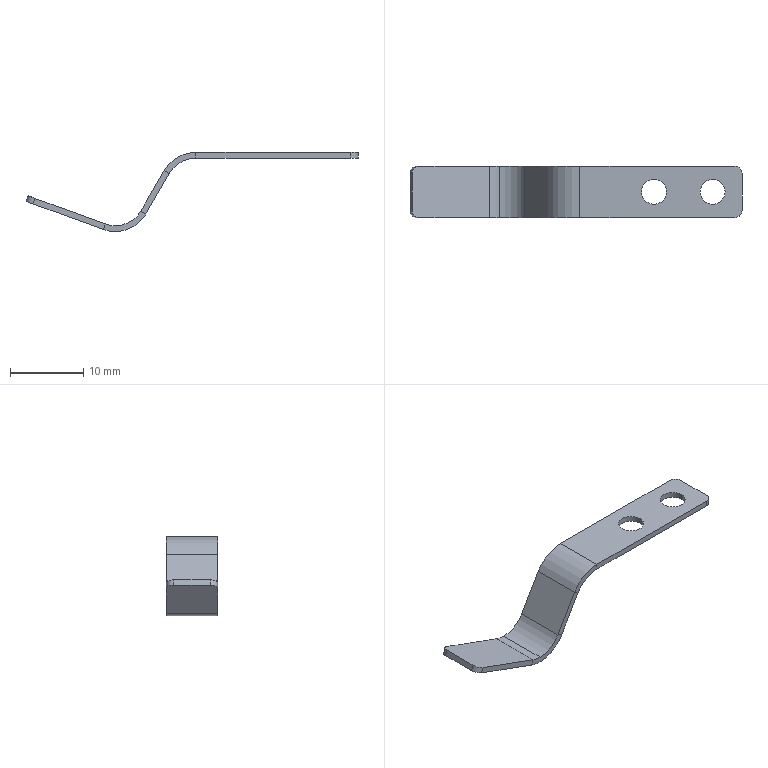Part | NX | features BREP 1 | 1 solid | 32 faces | box 45.274 x 7 x 10.8 mm | volume 268.431 mm3 | plane 18 | cylinder 14 | commonest cylinder face diameters 2 x4 3.4 x4 8 x2 9.6 x2 8.4 x1 10 x1
STEP:
#1=CARTESIAN_POINT('',(-2.3,0.,0.));
#2=VERTEX_POINT('',#1);
#3=CARTESIAN_POINT('',(-5.7,0.,0.));
#4=VERTEX_POINT('',#3);
#5=CARTESIAN_POINT('',(-4.,0.,0.));
#6=DIRECTION('',(0.,0.,-1.));
#7=DIRECTION('',(-1.,0.,0.));
#8=AXIS2_PLACEMENT_3D('',#5,#6,#7);
#9=CIRCLE('',#8,1.7);
#10=EDGE_CURVE('',#2,#4,#9,.T.);
#11=ORIENTED_EDGE('',*,*,#10,.F.);
#12=CARTESIAN_POINT('',(-2.3,0.,-0.8));
#13=VERTEX_POINT('',#12);
#14=CARTESIAN_POINT('',(-2.3,0.,-0.8));
#15=DIRECTION('',(0.,0.,-1.));
#16=VECTOR('',#15,1000.);
#17=LINE('',#14,#16);
#18=EDGE_CURVE('',#13,#2,#17,.F.);
#19=ORIENTED_EDGE('',*,*,#18,.F.);
#20=CARTESIAN_POINT('',(-5.7,0.,-0.8));
#21=VERTEX_POINT('',#20);
#22=CARTESIAN_POINT('',(-4.,0.,-0.8));
#23=DIRECTION('',(0.,0.,-1.));
#24=DIRECTION('',(-1.,0.,0.));
#25=AXIS2_PLACEMENT_3D('',#22,#23,#24);
#26=CIRCLE('',#25,1.7);
#27=EDGE_CURVE('',#13,#21,#26,.T.);
#28=ORIENTED_EDGE('',*,*,#27,.T.);
#29=CARTESIAN_POINT('',(-5.7,0.,-0.8));
#30=DIRECTION('',(0.,0.,-1.));
#31=VECTOR('',#30,1000.);
#32=LINE('',#29,#31);
#33=EDGE_CURVE('',#21,#4,#32,.F.);
#34=ORIENTED_EDGE('',*,*,#33,.T.);
#35=EDGE_LOOP('',(#11,#19,#28,#34));
#36=FACE_BOUND('',#35,.T.);
#37=CARTESIAN_POINT('',(-4.,0.,-0.8));
#38=DIRECTION('',(0.,0.,-1.));
#39=DIRECTION('',(1.,0.,0.));
#40=AXIS2_PLACEMENT_3D('',#37,#38,#39);
#41=CYLINDRICAL_SURFACE('',#40,1.7);
#42=ADVANCED_FACE('',(#36),#41,.F.);
#43=CARTESIAN_POINT('',(-10.3,0.,0.));
#44=VERTEX_POINT('',#43);
#45=CARTESIAN_POINT('',(-13.7,0.,0.));
#46=VERTEX_POINT('',#45);
#47=CARTESIAN_POINT('',(-12.,0.,0.));
#48=DIRECTION('',(0.,0.,-1.));
#49=DIRECTION('',(-1.,0.,0.));
#50=AXIS2_PLACEMENT_3D('',#47,#48,#49);
#51=CIRCLE('',#50,1.7);
#52=EDGE_CURVE('',#44,#46,#51,.T.);
#53=ORIENTED_EDGE('',*,*,#52,.F.);
#54=CARTESIAN_POINT('',(-10.3,0.,-0.8));
#55=VERTEX_POINT('',#54);
#56=CARTESIAN_POINT('',(-10.3,0.,-0.8));
#57=DIRECTION('',(0.,0.,-1.));
#58=VECTOR('',#57,1000.);
#59=LINE('',#56,#58);
#60=EDGE_CURVE('',#55,#44,#59,.F.);
#61=ORIENTED_EDGE('',*,*,#60,.F.);
#62=CARTESIAN_POINT('',(-13.7,0.,-0.8));
#63=VERTEX_POINT('',#62);
#64=CARTESIAN_POINT('',(-12.,0.,-0.8));
#65=DIRECTION('',(0.,0.,-1.));
#66=DIRECTION('',(-1.,0.,0.));
#67=AXIS2_PLACEMENT_3D('',#64,#65,#66);
#68=CIRCLE('',#67,1.7);
#69=EDGE_CURVE('',#55,#63,#68,.T.);
#70=ORIENTED_EDGE('',*,*,#69,.T.);
#71=CARTESIAN_POINT('',(-13.7,0.,-0.8));
#72=DIRECTION('',(0.,0.,-1.));
#73=VECTOR('',#72,1000.);
#74=LINE('',#71,#73);
#75=EDGE_CURVE('',#63,#46,#74,.F.);
#76=ORIENTED_EDGE('',*,*,#75,.T.);
#77=EDGE_LOOP('',(#53,#61,#70,#76));
#78=FACE_BOUND('',#77,.T.);
#79=CARTESIAN_POINT('',(-12.,0.,-0.8));
#80=DIRECTION('',(0.,0.,-1.));
#81=DIRECTION('',(1.,0.,0.));
#82=AXIS2_PLACEMENT_3D('',#79,#80,#81);
#83=CYLINDRICAL_SURFACE('',#82,1.7);
#84=ADVANCED_FACE('',(#78),#83,.F.);
#85=CARTESIAN_POINT('',(-33.083,3.5,-10.8));
#86=VERTEX_POINT('',#85);
#87=CARTESIAN_POINT('',(-34.725,3.5,-10.511));
#88=VERTEX_POINT('',#87);
#89=CARTESIAN_POINT('',(-33.083,3.5,-6.));
#90=DIRECTION('',(0.,1.,0.));
#91=DIRECTION('',(1.,0.,0.));
#92=AXIS2_PLACEMENT_3D('',#89,#90,#91);
#93=CIRCLE('',#92,4.8);
#94=EDGE_CURVE('',#86,#88,#93,.T.);
#95=ORIENTED_EDGE('',*,*,#94,.F.);
#96=CARTESIAN_POINT('',(-33.083,-3.5,-10.8));
#97=VERTEX_POINT('',#96);
#98=CARTESIAN_POINT('',(-33.083,3.5,-10.8));
#99=DIRECTION('',(0.,-1.,0.));
#100=VECTOR('',#99,1000.);
#101=LINE('',#98,#100);
#102=EDGE_CURVE('',#86,#97,#101,.T.);
#103=ORIENTED_EDGE('',*,*,#102,.T.);
#104=CARTESIAN_POINT('',(-34.725,-3.5,-10.511));
#105=VERTEX_POINT('',#104);
#106=CARTESIAN_POINT('',(-33.083,-3.5,-6.));
#107=DIRECTION('',(0.,1.,0.));
#108=DIRECTION('',(1.,0.,0.));
#109=AXIS2_PLACEMENT_3D('',#106,#107,#108);
#110=CIRCLE('',#109,4.8);
#111=EDGE_CURVE('',#97,#105,#110,.T.);
#112=ORIENTED_EDGE('',*,*,#111,.T.);
#113=CARTESIAN_POINT('',(-34.725,3.5,-10.511));
#114=DIRECTION('',(0.,-1.,0.));
#115=VECTOR('',#114,1000.);
#116=LINE('',#113,#115);
#117=EDGE_CURVE('',#88,#105,#116,.T.);
#118=ORIENTED_EDGE('',*,*,#117,.F.);
#119=EDGE_LOOP('',(#95,#103,#112,#118));
#120=FACE_BOUND('',#119,.T.);
#121=CARTESIAN_POINT('',(-33.083,3.5,-6.));
#122=DIRECTION('',(0.,-1.,0.));
#123=DIRECTION('',(0.,0.,1.));
#124=AXIS2_PLACEMENT_3D('',#121,#122,#123);
#125=CYLINDRICAL_SURFACE('',#124,4.8);
#126=ADVANCED_FACE('',(#120),#125,.T.);
#127=CARTESIAN_POINT('',(-29.619,3.5,-8.));
#128=VERTEX_POINT('',#127);
#129=CARTESIAN_POINT('',(-33.083,3.5,-10.));
#130=VERTEX_POINT('',#129);
#131=CARTESIAN_POINT('',(-33.083,3.5,-6.));
#132=DIRECTION('',(0.,1.,0.));
#133=DIRECTION('',(0.,0.,-1.));
#134=AXIS2_PLACEMENT_3D('',#131,#132,#133);
#135=CIRCLE('',#134,4.);
#136=EDGE_CURVE('',#128,#130,#135,.T.);
#137=ORIENTED_EDGE('',*,*,#136,.T.);
#138=CARTESIAN_POINT('',(-33.083,-3.5,-10.));
#139=VERTEX_POINT('',#138);
#140=CARTESIAN_POINT('',(-33.083,3.5,-10.));
#141=DIRECTION('',(0.,-1.,0.));
#142=VECTOR('',#141,1000.);
#143=LINE('',#140,#142);
#144=EDGE_CURVE('',#130,#139,#143,.T.);
#145=ORIENTED_EDGE('',*,*,#144,.T.);
#146=CARTESIAN_POINT('',(-29.619,-3.5,-8.));
#147=VERTEX_POINT('',#146);
#148=CARTESIAN_POINT('',(-33.083,-3.5,-6.));
#149=DIRECTION('',(0.,1.,0.));
#150=DIRECTION('',(0.,0.,-1.));
#151=AXIS2_PLACEMENT_3D('',#148,#149,#150);
#152=CIRCLE('',#151,4.);
#153=EDGE_CURVE('',#147,#139,#152,.T.);
#154=ORIENTED_EDGE('',*,*,#153,.F.);
#155=CARTESIAN_POINT('',(-29.619,3.5,-8.));
#156=DIRECTION('',(0.,-1.,0.));
#157=VECTOR('',#156,1000.);
#158=LINE('',#155,#157);
#159=EDGE_CURVE('',#128,#147,#158,.T.);
#160=ORIENTED_EDGE('',*,*,#159,.F.);
#161=EDGE_LOOP('',(#137,#145,#154,#160));
#162=FACE_BOUND('',#161,.T.);
#163=CARTESIAN_POINT('',(-33.083,3.5,-6.));
#164=DIRECTION('',(0.,-1.,0.));
#165=DIRECTION('',(0.,0.,1.));
#166=AXIS2_PLACEMENT_3D('',#163,#164,#165);
#167=CYLINDRICAL_SURFACE('',#166,4.);
#168=ADVANCED_FACE('',(#162),#167,.F.);
#169=CARTESIAN_POINT('',(-26.443,3.5,-2.5));
#170=VERTEX_POINT('',#169);
#171=CARTESIAN_POINT('',(-25.751,3.5,-2.9));
#172=VERTEX_POINT('',#171);
#173=CARTESIAN_POINT('',(-26.443,3.5,-2.5));
#174=DIRECTION('',(0.866,0.,-0.5));
#175=VECTOR('',#174,1000.);
#176=LINE('',#173,#175);
#177=EDGE_CURVE('',#170,#172,#176,.T.);
#178=ORIENTED_EDGE('',*,*,#177,.F.);
#179=CARTESIAN_POINT('',(-22.113,3.5,0.));
#180=VERTEX_POINT('',#179);
#181=CARTESIAN_POINT('',(-22.113,3.5,-5.));
#182=DIRECTION('',(0.,-1.,0.));
#183=DIRECTION('',(0.,0.,-1.));
#184=AXIS2_PLACEMENT_3D('',#181,#182,#183);
#185=CIRCLE('',#184,5.);
#186=EDGE_CURVE('',#180,#170,#185,.T.);
#187=ORIENTED_EDGE('',*,*,#186,.F.);
#188=CARTESIAN_POINT('',(-22.113,3.5,-0.8));
#189=VERTEX_POINT('',#188);
#190=CARTESIAN_POINT('',(-22.113,3.5,-0.8));
#191=DIRECTION('',(0.,0.,1.));
#192=VECTOR('',#191,1000.);
#193=LINE('',#190,#192);
#194=EDGE_CURVE('',#189,#180,#193,.T.);
#195=ORIENTED_EDGE('',*,*,#194,.F.);
#196=CARTESIAN_POINT('',(-22.113,3.5,-5.));
#197=DIRECTION('',(0.,-1.,0.));
#198=DIRECTION('',(1.,0.,0.));
#199=AXIS2_PLACEMENT_3D('',#196,#197,#198);
#200=CIRCLE('',#199,4.2);
#201=EDGE_CURVE('',#189,#172,#200,.T.);
#202=ORIENTED_EDGE('',*,*,#201,.T.);
#203=EDGE_LOOP('',(#178,#187,#195,#202));
#204=FACE_BOUND('',#203,.T.);
#205=CARTESIAN_POINT('',(-26.443,3.5,-2.5));
#206=DIRECTION('',(0.,1.,0.));
#207=DIRECTION('',(0.,0.,-1.));
#208=AXIS2_PLACEMENT_3D('',#205,#206,#207);
#209=PLANE('',#208);
#210=ADVANCED_FACE('',(#204),#209,.T.);
#211=CARTESIAN_POINT('',(-26.443,3.5,-2.5));
#212=DIRECTION('',(-0.5,0.,-0.866));
#213=VECTOR('',#212,1000.);
#214=LINE('',#211,#213);
#215=EDGE_CURVE('',#170,#128,#214,.T.);
#216=ORIENTED_EDGE('',*,*,#215,.F.);
#217=ORIENTED_EDGE('',*,*,#177,.T.);
#218=CARTESIAN_POINT('',(-28.926,3.5,-8.4));
#219=VERTEX_POINT('',#218);
#220=CARTESIAN_POINT('',(-25.751,3.5,-2.9));
#221=DIRECTION('',(-0.5,0.,-0.866));
#222=VECTOR('',#221,1000.);
#223=LINE('',#220,#222);
#224=EDGE_CURVE('',#172,#219,#223,.T.);
#225=ORIENTED_EDGE('',*,*,#224,.T.);
#226=CARTESIAN_POINT('',(-28.926,3.5,-8.4));
#227=DIRECTION('',(-0.866,0.,0.5));
#228=VECTOR('',#227,1000.);
#229=LINE('',#226,#228);
#230=EDGE_CURVE('',#219,#128,#229,.T.);
#231=ORIENTED_EDGE('',*,*,#230,.T.);
#232=EDGE_LOOP('',(#216,#217,#225,#231));
#233=FACE_BOUND('',#232,.T.);
#234=CARTESIAN_POINT('',(-22.113,3.5,-0.8));
#235=DIRECTION('',(0.,1.,0.));
#236=DIRECTION('',(0.,0.,-1.));
#237=AXIS2_PLACEMENT_3D('',#234,#235,#236);
#238=PLANE('',#237);
#239=ADVANCED_FACE('',(#233),#238,.T.);
#240=CARTESIAN_POINT('',(-22.113,-3.5,0.));
#241=VERTEX_POINT('',#240);
#242=CARTESIAN_POINT('',(-22.113,-3.5,-0.8));
#243=VERTEX_POINT('',#242);
#244=CARTESIAN_POINT('',(-22.113,-3.5,0.));
#245=DIRECTION('',(0.,0.,-1.));
#246=VECTOR('',#245,1000.);
#247=LINE('',#244,#246);
#248=EDGE_CURVE('',#241,#243,#247,.T.);
#249=ORIENTED_EDGE('',*,*,#248,.F.);
#250=CARTESIAN_POINT('',(-26.443,-3.5,-2.5));
#251=VERTEX_POINT('',#250);
#252=CARTESIAN_POINT('',(-22.113,-3.5,-5.));
#253=DIRECTION('',(0.,-1.,0.));
#254=DIRECTION('',(0.,0.,-1.));
#255=AXIS2_PLACEMENT_3D('',#252,#253,#254);
#256=CIRCLE('',#255,5.);
#257=EDGE_CURVE('',#241,#251,#256,.T.);
#258=ORIENTED_EDGE('',*,*,#257,.T.);
#259=CARTESIAN_POINT('',(-25.751,-3.5,-2.9));
#260=VERTEX_POINT('',#259);
#261=CARTESIAN_POINT('',(-25.751,-3.5,-2.9));
#262=DIRECTION('',(-0.866,0.,0.5));
#263=VECTOR('',#262,1000.);
#264=LINE('',#261,#263);
#265=EDGE_CURVE('',#260,#251,#264,.T.);
#266=ORIENTED_EDGE('',*,*,#265,.F.);
#267=CARTESIAN_POINT('',(-22.113,-3.5,-5.));
#268=DIRECTION('',(0.,-1.,0.));
#269=DIRECTION('',(1.,0.,0.));
#270=AXIS2_PLACEMENT_3D('',#267,#268,#269);
#271=CIRCLE('',#270,4.2);
#272=EDGE_CURVE('',#243,#260,#271,.T.);
#273=ORIENTED_EDGE('',*,*,#272,.F.);
#274=EDGE_LOOP('',(#249,#258,#266,#273));
#275=FACE_BOUND('',#274,.T.);
#276=CARTESIAN_POINT('',(-22.113,-3.5,0.));
#277=DIRECTION('',(0.,-1.,0.));
#278=DIRECTION('',(0.,0.,1.));
#279=AXIS2_PLACEMENT_3D('',#276,#277,#278);
#280=PLANE('',#279);
#281=ADVANCED_FACE('',(#275),#280,.T.);
#282=CARTESIAN_POINT('',(-1.,-3.5,-0.8));
#283=VERTEX_POINT('',#282);
#284=CARTESIAN_POINT('',(0.,-3.5,-0.8));
#285=DIRECTION('',(-1.,0.,0.));
#286=VECTOR('',#285,1000.);
#287=LINE('',#284,#286);
#288=EDGE_CURVE('',#283,#243,#287,.T.);
#289=ORIENTED_EDGE('',*,*,#288,.F.);
#290=CARTESIAN_POINT('',(-1.,-3.5,0.));
#291=VERTEX_POINT('',#290);
#292=CARTESIAN_POINT('',(-1.,-3.5,-2.9));
#293=DIRECTION('',(0.,0.,1.));
#294=VECTOR('',#293,1000.);
#295=LINE('',#292,#294);
#296=EDGE_CURVE('',#283,#291,#295,.T.);
#297=ORIENTED_EDGE('',*,*,#296,.T.);
#298=CARTESIAN_POINT('',(0.,-3.5,0.));
#299=DIRECTION('',(-1.,0.,0.));
#300=VECTOR('',#299,1000.);
#301=LINE('',#298,#300);
#302=EDGE_CURVE('',#291,#241,#301,.T.);
#303=ORIENTED_EDGE('',*,*,#302,.T.);
#304=ORIENTED_EDGE('',*,*,#248,.T.);
#305=EDGE_LOOP('',(#289,#297,#303,#304));
#306=FACE_BOUND('',#305,.T.);
#307=CARTESIAN_POINT('',(-25.751,-3.5,-2.9));
#308=DIRECTION('',(0.,-1.,0.));
#309=DIRECTION('',(0.,0.,1.));
#310=AXIS2_PLACEMENT_3D('',#307,#308,#309);
#311=PLANE('',#310);
#312=ADVANCED_FACE('',(#306),#311,.T.);
#313=CARTESIAN_POINT('',(-34.451,3.5,-9.759));
#314=VERTEX_POINT('',#313);
#315=CARTESIAN_POINT('',(-34.451,3.5,-9.759));
#316=DIRECTION('',(-0.342,0.,-0.9397));
#317=VECTOR('',#316,1000.);
#318=LINE('',#315,#317);
#319=EDGE_CURVE('',#314,#88,#318,.T.);
#320=ORIENTED_EDGE('',*,*,#319,.F.);
#321=CARTESIAN_POINT('',(-33.083,3.5,-6.));
#322=DIRECTION('',(0.,1.,0.));
#323=DIRECTION('',(0.,0.,-1.));
#324=AXIS2_PLACEMENT_3D('',#321,#322,#323);
#325=CIRCLE('',#324,4.);
#326=EDGE_CURVE('',#130,#314,#325,.T.);
#327=ORIENTED_EDGE('',*,*,#326,.F.);
#328=ORIENTED_EDGE('',*,*,#136,.F.);
#329=ORIENTED_EDGE('',*,*,#230,.F.);
#330=CARTESIAN_POINT('',(-33.083,3.5,-6.));
#331=DIRECTION('',(0.,1.,0.));
#332=DIRECTION('',(1.,0.,0.));
#333=AXIS2_PLACEMENT_3D('',#330,#331,#332);
#334=CIRCLE('',#333,4.8);
#335=EDGE_CURVE('',#219,#86,#334,.T.);
#336=ORIENTED_EDGE('',*,*,#335,.T.);
#337=ORIENTED_EDGE('',*,*,#94,.T.);
#338=EDGE_LOOP('',(#320,#327,#328,#329,#336,#337));
#339=FACE_BOUND('',#338,.T.);
#340=CARTESIAN_POINT('',(-34.451,3.5,-9.759));
#341=DIRECTION('',(0.,1.,0.));
#342=DIRECTION('',(0.,0.,-1.));
#343=AXIS2_PLACEMENT_3D('',#340,#341,#342);
#344=PLANE('',#343);
#345=ADVANCED_FACE('',(#339),#344,.T.);
#346=CARTESIAN_POINT('',(-44.334,3.5,-7.013));
#347=VERTEX_POINT('',#346);
#348=CARTESIAN_POINT('',(-34.725,3.5,-10.511));
#349=DIRECTION('',(-0.9397,0.,0.342));
#350=VECTOR('',#349,1000.);
#351=LINE('',#348,#350);
#352=EDGE_CURVE('',#88,#347,#351,.T.);
#353=ORIENTED_EDGE('',*,*,#352,.T.);
#354=CARTESIAN_POINT('',(-44.06,3.5,-6.261));
#355=VERTEX_POINT('',#354);
#356=CARTESIAN_POINT('',(-42.977,3.5,-3.286));
#357=DIRECTION('',(0.342,0.,0.9397));
#358=VECTOR('',#357,1000.);
#359=LINE('',#356,#358);
#360=EDGE_CURVE('',#347,#355,#359,.T.);
#361=ORIENTED_EDGE('',*,*,#360,.T.);
#362=CARTESIAN_POINT('',(-34.451,3.5,-9.759));
#363=DIRECTION('',(-0.9397,0.,0.342));
#364=VECTOR('',#363,1000.);
#365=LINE('',#362,#364);
#366=EDGE_CURVE('',#314,#355,#365,.T.);
#367=ORIENTED_EDGE('',*,*,#366,.F.);
#368=ORIENTED_EDGE('',*,*,#319,.T.);
#369=EDGE_LOOP('',(#353,#361,#367,#368));
#370=FACE_BOUND('',#369,.T.);
#371=CARTESIAN_POINT('',(-28.926,3.5,-8.4));
#372=DIRECTION('',(0.,1.,0.));
#373=DIRECTION('',(0.,0.,-1.));
#374=AXIS2_PLACEMENT_3D('',#371,#372,#373);
#375=PLANE('',#374);
#376=ADVANCED_FACE('',(#370),#375,.T.);
#377=CARTESIAN_POINT('',(-28.926,-3.5,-8.4));
#378=VERTEX_POINT('',#377);
#379=CARTESIAN_POINT('',(-29.619,-3.5,-8.));
#380=DIRECTION('',(0.866,0.,-0.5));
#381=VECTOR('',#380,1000.);
#382=LINE('',#379,#381);
#383=EDGE_CURVE('',#147,#378,#382,.T.);
#384=ORIENTED_EDGE('',*,*,#383,.F.);
#385=ORIENTED_EDGE('',*,*,#153,.T.);
#386=CARTESIAN_POINT('',(-34.451,-3.5,-9.759));
#387=VERTEX_POINT('',#386);
#388=CARTESIAN_POINT('',(-33.083,-3.5,-6.));
#389=DIRECTION('',(0.,1.,0.));
#390=DIRECTION('',(0.,0.,-1.));
#391=AXIS2_PLACEMENT_3D('',#388,#389,#390);
#392=CIRCLE('',#391,4.);
#393=EDGE_CURVE('',#139,#387,#392,.T.);
#394=ORIENTED_EDGE('',*,*,#393,.T.);
#395=CARTESIAN_POINT('',(-34.725,-3.5,-10.511));
#396=DIRECTION('',(0.342,0.,0.9397));
#397=VECTOR('',#396,1000.);
#398=LINE('',#395,#397);
#399=EDGE_CURVE('',#105,#387,#398,.T.);
#400=ORIENTED_EDGE('',*,*,#399,.F.);
#401=ORIENTED_EDGE('',*,*,#111,.F.);
#402=CARTESIAN_POINT('',(-33.083,-3.5,-6.));
#403=DIRECTION('',(0.,1.,0.));
#404=DIRECTION('',(1.,0.,0.));
#405=AXIS2_PLACEMENT_3D('',#402,#403,#404);
#406=CIRCLE('',#405,4.8);
#407=EDGE_CURVE('',#378,#97,#406,.T.);
#408=ORIENTED_EDGE('',*,*,#407,.F.);
#409=EDGE_LOOP('',(#384,#385,#394,#400,#401,#408));
#410=FACE_BOUND('',#409,.T.);
#411=CARTESIAN_POINT('',(-29.619,-3.5,-8.));
#412=DIRECTION('',(0.,-1.,0.));
#413=DIRECTION('',(0.,0.,1.));
#414=AXIS2_PLACEMENT_3D('',#411,#412,#413);
#415=PLANE('',#414);
#416=ADVANCED_FACE('',(#410),#415,.T.);
#417=CARTESIAN_POINT('',(-26.443,-3.5,-2.5));
#418=DIRECTION('',(-0.5,0.,-0.866));
#419=VECTOR('',#418,1000.);
#420=LINE('',#417,#419);
#421=EDGE_CURVE('',#251,#147,#420,.T.);
#422=ORIENTED_EDGE('',*,*,#421,.T.);
#423=ORIENTED_EDGE('',*,*,#383,.T.);
#424=CARTESIAN_POINT('',(-25.751,-3.5,-2.9));
#425=DIRECTION('',(-0.5,0.,-0.866));
#426=VECTOR('',#425,1000.);
#427=LINE('',#424,#426);
#428=EDGE_CURVE('',#260,#378,#427,.T.);
#429=ORIENTED_EDGE('',*,*,#428,.F.);
#430=ORIENTED_EDGE('',*,*,#265,.T.);
#431=EDGE_LOOP('',(#422,#423,#429,#430));
#432=FACE_BOUND('',#431,.T.);
#433=CARTESIAN_POINT('',(-34.725,-3.5,-10.511));
#434=DIRECTION('',(0.,-1.,0.));
#435=DIRECTION('',(0.,0.,1.));
#436=AXIS2_PLACEMENT_3D('',#433,#434,#435);
#437=PLANE('',#436);
#438=ADVANCED_FACE('',(#432),#437,.T.);
#439=CARTESIAN_POINT('',(-44.334,-3.5,-7.013));
#440=VERTEX_POINT('',#439);
#441=CARTESIAN_POINT('',(-34.725,-3.5,-10.511));
#442=DIRECTION('',(-0.9397,0.,0.342));
#443=VECTOR('',#442,1000.);
#444=LINE('',#441,#443);
#445=EDGE_CURVE('',#105,#440,#444,.T.);
#446=ORIENTED_EDGE('',*,*,#445,.T.);
#447=CARTESIAN_POINT('',(-45.274,-2.5,-6.671));
#448=VERTEX_POINT('',#447);
#449=CARTESIAN_POINT('',(-44.334,-2.5,-7.013));
#450=DIRECTION('',(-0.342,0.,-0.9397));
#451=DIRECTION('',(0.9397,0.,-0.342));
#452=AXIS2_PLACEMENT_3D('',#449,#450,#451);
#453=CIRCLE('',#452,1.);
#454=EDGE_CURVE('',#440,#448,#453,.T.);
#455=ORIENTED_EDGE('',*,*,#454,.T.);
#456=CARTESIAN_POINT('',(-45.274,2.5,-6.671));
#457=VERTEX_POINT('',#456);
#458=CARTESIAN_POINT('',(-45.274,3.5,-6.671));
#459=DIRECTION('',(0.,-1.,0.));
#460=VECTOR('',#459,1000.);
#461=LINE('',#458,#460);
#462=EDGE_CURVE('',#457,#448,#461,.T.);
#463=ORIENTED_EDGE('',*,*,#462,.F.);
#464=CARTESIAN_POINT('',(-44.334,2.5,-7.013));
#465=DIRECTION('',(-0.342,0.,-0.9397));
#466=DIRECTION('',(0.9397,0.,-0.342));
#467=AXIS2_PLACEMENT_3D('',#464,#465,#466);
#468=CIRCLE('',#467,1.);
#469=EDGE_CURVE('',#457,#347,#468,.T.);
#470=ORIENTED_EDGE('',*,*,#469,.T.);
#471=ORIENTED_EDGE('',*,*,#352,.F.);
#472=ORIENTED_EDGE('',*,*,#117,.T.);
#473=EDGE_LOOP('',(#446,#455,#463,#470,#471,#472));
#474=FACE_BOUND('',#473,.T.);
#475=CARTESIAN_POINT('',(-34.725,3.5,-10.511));
#476=DIRECTION('',(0.342,0.,0.9397));
#477=DIRECTION('',(-0.9397,0.,0.342));
#478=AXIS2_PLACEMENT_3D('',#475,#476,#477);
#479=PLANE('',#478);
#480=ADVANCED_FACE('',(#474),#479,.F.);
#481=ORIENTED_EDGE('',*,*,#462,.T.);
#482=CARTESIAN_POINT('',(-45.,-2.5,-5.919));
#483=VERTEX_POINT('',#482);
#484=CARTESIAN_POINT('',(-45.,-2.5,-5.919));
#485=DIRECTION('',(0.342,0.,0.9397));
#486=VECTOR('',#485,1000.);
#487=LINE('',#484,#486);
#488=EDGE_CURVE('',#448,#483,#487,.T.);
#489=ORIENTED_EDGE('',*,*,#488,.T.);
#490=CARTESIAN_POINT('',(-45.,2.5,-5.919));
#491=VERTEX_POINT('',#490);
#492=CARTESIAN_POINT('',(-45.,3.5,-5.919));
#493=DIRECTION('',(0.,-1.,0.));
#494=VECTOR('',#493,1000.);
#495=LINE('',#492,#494);
#496=EDGE_CURVE('',#491,#483,#495,.T.);
#497=ORIENTED_EDGE('',*,*,#496,.F.);
#498=CARTESIAN_POINT('',(-45.,2.5,-5.919));
#499=DIRECTION('',(-0.342,0.,-0.9397));
#500=VECTOR('',#499,1000.);
#501=LINE('',#498,#500);
#502=EDGE_CURVE('',#491,#457,#501,.T.);
#503=ORIENTED_EDGE('',*,*,#502,.T.);
#504=EDGE_LOOP('',(#481,#489,#497,#503));
#505=FACE_BOUND('',#504,.T.);
#506=CARTESIAN_POINT('',(-45.,3.5,-5.919));
#507=DIRECTION('',(-0.9397,0.,0.342));
#508=DIRECTION('',(-0.342,0.,-0.9397));
#509=AXIS2_PLACEMENT_3D('',#506,#507,#508);
#510=PLANE('',#509);
#511=ADVANCED_FACE('',(#505),#510,.T.);
#512=ORIENTED_EDGE('',*,*,#496,.T.);
#513=CARTESIAN_POINT('',(-44.06,-3.5,-6.261));
#514=VERTEX_POINT('',#513);
#515=CARTESIAN_POINT('',(-44.06,-2.5,-6.261));
#516=DIRECTION('',(0.342,0.,0.9397));
#517=DIRECTION('',(0.9397,0.,-0.342));
#518=AXIS2_PLACEMENT_3D('',#515,#516,#517);
#519=CIRCLE('',#518,1.);
#520=EDGE_CURVE('',#483,#514,#519,.T.);
#521=ORIENTED_EDGE('',*,*,#520,.T.);
#522=CARTESIAN_POINT('',(-34.451,-3.5,-9.759));
#523=DIRECTION('',(-0.9397,0.,0.342));
#524=VECTOR('',#523,1000.);
#525=LINE('',#522,#524);
#526=EDGE_CURVE('',#387,#514,#525,.T.);
#527=ORIENTED_EDGE('',*,*,#526,.F.);
#528=CARTESIAN_POINT('',(-34.451,3.5,-9.759));
#529=DIRECTION('',(0.,-1.,0.));
#530=VECTOR('',#529,1000.);
#531=LINE('',#528,#530);
#532=EDGE_CURVE('',#314,#387,#531,.T.);
#533=ORIENTED_EDGE('',*,*,#532,.F.);
#534=ORIENTED_EDGE('',*,*,#366,.T.);
#535=CARTESIAN_POINT('',(-44.06,2.5,-6.261));
#536=DIRECTION('',(0.342,0.,0.9397));
#537=DIRECTION('',(0.9397,0.,-0.342));
#538=AXIS2_PLACEMENT_3D('',#535,#536,#537);
#539=CIRCLE('',#538,1.);
#540=EDGE_CURVE('',#355,#491,#539,.T.);
#541=ORIENTED_EDGE('',*,*,#540,.T.);
#542=EDGE_LOOP('',(#512,#521,#527,#533,#534,#541));
#543=FACE_BOUND('',#542,.T.);
#544=CARTESIAN_POINT('',(-34.451,3.5,-9.759));
#545=DIRECTION('',(0.342,0.,0.9397));
#546=DIRECTION('',(-0.9397,0.,0.342));
#547=AXIS2_PLACEMENT_3D('',#544,#545,#546);
#548=PLANE('',#547);
#549=ADVANCED_FACE('',(#543),#548,.T.);
#550=ORIENTED_EDGE('',*,*,#144,.F.);
#551=ORIENTED_EDGE('',*,*,#326,.T.);
#552=ORIENTED_EDGE('',*,*,#532,.T.);
#553=ORIENTED_EDGE('',*,*,#393,.F.);
#554=EDGE_LOOP('',(#550,#551,#552,#553));
#555=FACE_BOUND('',#554,.T.);
#556=CARTESIAN_POINT('',(-33.083,3.5,-6.));
#557=DIRECTION('',(0.,-1.,0.));
#558=DIRECTION('',(0.,0.,1.));
#559=AXIS2_PLACEMENT_3D('',#556,#557,#558);
#560=CYLINDRICAL_SURFACE('',#559,4.);
#561=ADVANCED_FACE('',(#555),#560,.F.);
#562=ORIENTED_EDGE('',*,*,#421,.F.);
#563=CARTESIAN_POINT('',(-26.443,3.5,-2.5));
#564=DIRECTION('',(0.,-1.,0.));
#565=VECTOR('',#564,1000.);
#566=LINE('',#563,#565);
#567=EDGE_CURVE('',#170,#251,#566,.T.);
#568=ORIENTED_EDGE('',*,*,#567,.F.);
#569=ORIENTED_EDGE('',*,*,#215,.T.);
#570=ORIENTED_EDGE('',*,*,#159,.T.);
#571=EDGE_LOOP('',(#562,#568,#569,#570));
#572=FACE_BOUND('',#571,.T.);
#573=CARTESIAN_POINT('',(-26.443,3.5,-2.5));
#574=DIRECTION('',(-0.866,0.,0.5));
#575=DIRECTION('',(-0.5,0.,-0.866));
#576=AXIS2_PLACEMENT_3D('',#573,#574,#575);
#577=PLANE('',#576);
#578=ADVANCED_FACE('',(#572),#577,.T.);
#579=ORIENTED_EDGE('',*,*,#257,.F.);
#580=CARTESIAN_POINT('',(-22.113,3.5,0.));
#581=DIRECTION('',(0.,-1.,0.));
#582=VECTOR('',#581,1000.);
#583=LINE('',#580,#582);
#584=EDGE_CURVE('',#180,#241,#583,.T.);
#585=ORIENTED_EDGE('',*,*,#584,.F.);
#586=ORIENTED_EDGE('',*,*,#186,.T.);
#587=ORIENTED_EDGE('',*,*,#567,.T.);
#588=EDGE_LOOP('',(#579,#585,#586,#587));
#589=FACE_BOUND('',#588,.T.);
#590=CARTESIAN_POINT('',(-22.113,3.5,-5.));
#591=DIRECTION('',(0.,-1.,0.));
#592=DIRECTION('',(0.,0.,1.));
#593=AXIS2_PLACEMENT_3D('',#590,#591,#592);
#594=CYLINDRICAL_SURFACE('',#593,5.);
#595=ADVANCED_FACE('',(#589),#594,.T.);
#596=CARTESIAN_POINT('',(-4.,0.,0.));
#597=DIRECTION('',(0.,0.,-1.));
#598=DIRECTION('',(-1.,0.,0.));
#599=AXIS2_PLACEMENT_3D('',#596,#597,#598);
#600=CIRCLE('',#599,1.7);
#601=EDGE_CURVE('',#4,#2,#600,.T.);
#602=ORIENTED_EDGE('',*,*,#601,.T.);
#603=ORIENTED_EDGE('',*,*,#10,.T.);
#604=EDGE_LOOP('',(#602,#603));
#605=FACE_BOUND('',#604,.T.);
#606=CARTESIAN_POINT('',(-12.,0.,0.));
#607=DIRECTION('',(0.,0.,-1.));
#608=DIRECTION('',(-1.,0.,0.));
#609=AXIS2_PLACEMENT_3D('',#606,#607,#608);
#610=CIRCLE('',#609,1.7);
#611=EDGE_CURVE('',#46,#44,#610,.T.);
#612=ORIENTED_EDGE('',*,*,#611,.T.);
#613=ORIENTED_EDGE('',*,*,#52,.T.);
#614=EDGE_LOOP('',(#612,#613));
#615=FACE_BOUND('',#614,.T.);
#616=ORIENTED_EDGE('',*,*,#302,.F.);
#617=CARTESIAN_POINT('',(0.,-2.5,0.));
#618=VERTEX_POINT('',#617);
#619=CARTESIAN_POINT('',(-1.,-2.5,0.));
#620=DIRECTION('',(0.,0.,1.));
#621=DIRECTION('',(1.,0.,0.));
#622=AXIS2_PLACEMENT_3D('',#619,#620,#621);
#623=CIRCLE('',#622,1.);
#624=EDGE_CURVE('',#291,#618,#623,.T.);
#625=ORIENTED_EDGE('',*,*,#624,.T.);
#626=CARTESIAN_POINT('',(0.,2.5,0.));
#627=VERTEX_POINT('',#626);
#628=CARTESIAN_POINT('',(0.,3.5,0.));
#629=DIRECTION('',(0.,-1.,0.));
#630=VECTOR('',#629,1000.);
#631=LINE('',#628,#630);
#632=EDGE_CURVE('',#627,#618,#631,.T.);
#633=ORIENTED_EDGE('',*,*,#632,.F.);
#634=CARTESIAN_POINT('',(-1.,3.5,0.));
#635=VERTEX_POINT('',#634);
#636=CARTESIAN_POINT('',(-1.,2.5,0.));
#637=DIRECTION('',(0.,0.,1.));
#638=DIRECTION('',(1.,0.,0.));
#639=AXIS2_PLACEMENT_3D('',#636,#637,#638);
#640=CIRCLE('',#639,1.);
#641=EDGE_CURVE('',#627,#635,#640,.T.);
#642=ORIENTED_EDGE('',*,*,#641,.T.);
#643=CARTESIAN_POINT('',(0.,3.5,0.));
#644=DIRECTION('',(-1.,0.,0.));
#645=VECTOR('',#644,1000.);
#646=LINE('',#643,#645);
#647=EDGE_CURVE('',#635,#180,#646,.T.);
#648=ORIENTED_EDGE('',*,*,#647,.T.);
#649=ORIENTED_EDGE('',*,*,#584,.T.);
#650=EDGE_LOOP('',(#616,#625,#633,#642,#648,#649));
#651=FACE_BOUND('',#650,.T.);
#652=CARTESIAN_POINT('',(0.,3.5,0.));
#653=DIRECTION('',(0.,0.,1.));
#654=DIRECTION('',(-1.,0.,0.));
#655=AXIS2_PLACEMENT_3D('',#652,#653,#654);
#656=PLANE('',#655);
#657=ADVANCED_FACE('',(#605,#615,#651),#656,.T.);
#658=ORIENTED_EDGE('',*,*,#632,.T.);
#659=CARTESIAN_POINT('',(0.,-2.5,-0.8));
#660=VERTEX_POINT('',#659);
#661=CARTESIAN_POINT('',(0.,-2.5,-0.8));
#662=DIRECTION('',(0.,0.,-1.));
#663=VECTOR('',#662,1000.);
#664=LINE('',#661,#663);
#665=EDGE_CURVE('',#618,#660,#664,.T.);
#666=ORIENTED_EDGE('',*,*,#665,.T.);
#667=CARTESIAN_POINT('',(0.,2.5,-0.8));
#668=VERTEX_POINT('',#667);
#669=CARTESIAN_POINT('',(0.,3.5,-0.8));
#670=DIRECTION('',(0.,-1.,0.));
#671=VECTOR('',#670,1000.);
#672=LINE('',#669,#671);
#673=EDGE_CURVE('',#668,#660,#672,.T.);
#674=ORIENTED_EDGE('',*,*,#673,.F.);
#675=CARTESIAN_POINT('',(0.,2.5,-0.8));
#676=DIRECTION('',(0.,0.,1.));
#677=VECTOR('',#676,1000.);
#678=LINE('',#675,#677);
#679=EDGE_CURVE('',#668,#627,#678,.T.);
#680=ORIENTED_EDGE('',*,*,#679,.T.);
#681=EDGE_LOOP('',(#658,#666,#674,#680));
#682=FACE_BOUND('',#681,.T.);
#683=CARTESIAN_POINT('',(0.,3.5,-0.8));
#684=DIRECTION('',(1.,0.,0.));
#685=DIRECTION('',(0.,0.,1.));
#686=AXIS2_PLACEMENT_3D('',#683,#684,#685);
#687=PLANE('',#686);
#688=ADVANCED_FACE('',(#682),#687,.T.);
#689=CARTESIAN_POINT('',(-4.,0.,-0.8));
#690=DIRECTION('',(0.,0.,-1.));
#691=DIRECTION('',(-1.,0.,0.));
#692=AXIS2_PLACEMENT_3D('',#689,#690,#691);
#693=CIRCLE('',#692,1.7);
#694=EDGE_CURVE('',#21,#13,#693,.T.);
#695=ORIENTED_EDGE('',*,*,#694,.F.);
#696=ORIENTED_EDGE('',*,*,#27,.F.);
#697=EDGE_LOOP('',(#695,#696));
#698=FACE_BOUND('',#697,.T.);
#699=CARTESIAN_POINT('',(-12.,0.,-0.8));
#700=DIRECTION('',(0.,0.,-1.));
#701=DIRECTION('',(-1.,0.,0.));
#702=AXIS2_PLACEMENT_3D('',#699,#700,#701);
#703=CIRCLE('',#702,1.7);
#704=EDGE_CURVE('',#63,#55,#703,.T.);
#705=ORIENTED_EDGE('',*,*,#704,.F.);
#706=ORIENTED_EDGE('',*,*,#69,.F.);
#707=EDGE_LOOP('',(#705,#706));
#708=FACE_BOUND('',#707,.T.);
#709=ORIENTED_EDGE('',*,*,#673,.T.);
#710=CARTESIAN_POINT('',(-1.,-2.5,-0.8));
#711=DIRECTION('',(0.,0.,-1.));
#712=DIRECTION('',(1.,0.,0.));
#713=AXIS2_PLACEMENT_3D('',#710,#711,#712);
#714=CIRCLE('',#713,1.);
#715=EDGE_CURVE('',#660,#283,#714,.T.);
#716=ORIENTED_EDGE('',*,*,#715,.T.);
#717=ORIENTED_EDGE('',*,*,#288,.T.);
#718=CARTESIAN_POINT('',(-22.113,3.5,-0.8));
#719=DIRECTION('',(0.,-1.,0.));
#720=VECTOR('',#719,1000.);
#721=LINE('',#718,#720);
#722=EDGE_CURVE('',#189,#243,#721,.T.);
#723=ORIENTED_EDGE('',*,*,#722,.F.);
#724=CARTESIAN_POINT('',(-1.,3.5,-0.8));
#725=VERTEX_POINT('',#724);
#726=CARTESIAN_POINT('',(0.,3.5,-0.8));
#727=DIRECTION('',(-1.,0.,0.));
#728=VECTOR('',#727,1000.);
#729=LINE('',#726,#728);
#730=EDGE_CURVE('',#725,#189,#729,.T.);
#731=ORIENTED_EDGE('',*,*,#730,.F.);
#732=CARTESIAN_POINT('',(-1.,2.5,-0.8));
#733=DIRECTION('',(0.,0.,-1.));
#734=DIRECTION('',(1.,0.,0.));
#735=AXIS2_PLACEMENT_3D('',#732,#733,#734);
#736=CIRCLE('',#735,1.);
#737=EDGE_CURVE('',#725,#668,#736,.T.);
#738=ORIENTED_EDGE('',*,*,#737,.T.);
#739=EDGE_LOOP('',(#709,#716,#717,#723,#731,#738));
#740=FACE_BOUND('',#739,.T.);
#741=CARTESIAN_POINT('',(0.,3.5,-0.8));
#742=DIRECTION('',(0.,0.,1.));
#743=DIRECTION('',(-1.,0.,0.));
#744=AXIS2_PLACEMENT_3D('',#741,#742,#743);
#745=PLANE('',#744);
#746=ADVANCED_FACE('',(#698,#708,#740),#745,.F.);
#747=ORIENTED_EDGE('',*,*,#272,.T.);
#748=CARTESIAN_POINT('',(-25.751,3.5,-2.9));
#749=DIRECTION('',(0.,-1.,0.));
#750=VECTOR('',#749,1000.);
#751=LINE('',#748,#750);
#752=EDGE_CURVE('',#172,#260,#751,.T.);
#753=ORIENTED_EDGE('',*,*,#752,.F.);
#754=ORIENTED_EDGE('',*,*,#201,.F.);
#755=ORIENTED_EDGE('',*,*,#722,.T.);
#756=EDGE_LOOP('',(#747,#753,#754,#755));
#757=FACE_BOUND('',#756,.T.);
#758=CARTESIAN_POINT('',(-22.113,3.5,-5.));
#759=DIRECTION('',(0.,-1.,0.));
#760=DIRECTION('',(0.,0.,1.));
#761=AXIS2_PLACEMENT_3D('',#758,#759,#760);
#762=CYLINDRICAL_SURFACE('',#761,4.2);
#763=ADVANCED_FACE('',(#757),#762,.F.);
#764=ORIENTED_EDGE('',*,*,#428,.T.);
#765=CARTESIAN_POINT('',(-28.926,3.5,-8.4));
#766=DIRECTION('',(0.,-1.,0.));
#767=VECTOR('',#766,1000.);
#768=LINE('',#765,#767);
#769=EDGE_CURVE('',#219,#378,#768,.T.);
#770=ORIENTED_EDGE('',*,*,#769,.F.);
#771=ORIENTED_EDGE('',*,*,#224,.F.);
#772=ORIENTED_EDGE('',*,*,#752,.T.);
#773=EDGE_LOOP('',(#764,#770,#771,#772));
#774=FACE_BOUND('',#773,.T.);
#775=CARTESIAN_POINT('',(-25.751,3.5,-2.9));
#776=DIRECTION('',(-0.866,0.,0.5));
#777=DIRECTION('',(-0.5,0.,-0.866));
#778=AXIS2_PLACEMENT_3D('',#775,#776,#777);
#779=PLANE('',#778);
#780=ADVANCED_FACE('',(#774),#779,.F.);
#781=ORIENTED_EDGE('',*,*,#102,.F.);
#782=ORIENTED_EDGE('',*,*,#335,.F.);
#783=ORIENTED_EDGE('',*,*,#769,.T.);
#784=ORIENTED_EDGE('',*,*,#407,.T.);
#785=EDGE_LOOP('',(#781,#782,#783,#784));
#786=FACE_BOUND('',#785,.T.);
#787=CARTESIAN_POINT('',(-33.083,3.5,-6.));
#788=DIRECTION('',(0.,-1.,0.));
#789=DIRECTION('',(0.,0.,1.));
#790=AXIS2_PLACEMENT_3D('',#787,#788,#789);
#791=CYLINDRICAL_SURFACE('',#790,4.8);
#792=ADVANCED_FACE('',(#786),#791,.T.);
#793=ORIENTED_EDGE('',*,*,#647,.F.);
#794=CARTESIAN_POINT('',(-1.,3.5,-6.));
#795=DIRECTION('',(0.,0.,-1.));
#796=VECTOR('',#795,1000.);
#797=LINE('',#794,#796);
#798=EDGE_CURVE('',#635,#725,#797,.T.);
#799=ORIENTED_EDGE('',*,*,#798,.T.);
#800=ORIENTED_EDGE('',*,*,#730,.T.);
#801=ORIENTED_EDGE('',*,*,#194,.T.);
#802=EDGE_LOOP('',(#793,#799,#800,#801));
#803=FACE_BOUND('',#802,.T.);
#804=CARTESIAN_POINT('',(-33.083,3.5,-6.));
#805=DIRECTION('',(0.,1.,0.));
#806=DIRECTION('',(-1.,0.,0.));
#807=AXIS2_PLACEMENT_3D('',#804,#805,#806);
#808=PLANE('',#807);
#809=ADVANCED_FACE('',(#803),#808,.T.);
#810=ORIENTED_EDGE('',*,*,#526,.T.);
#811=CARTESIAN_POINT('',(-44.334,-3.5,-7.013));
#812=DIRECTION('',(-0.342,0.,-0.9397));
#813=VECTOR('',#812,1000.);
#814=LINE('',#811,#813);
#815=EDGE_CURVE('',#514,#440,#814,.T.);
#816=ORIENTED_EDGE('',*,*,#815,.T.);
#817=ORIENTED_EDGE('',*,*,#445,.F.);
#818=ORIENTED_EDGE('',*,*,#399,.T.);
#819=EDGE_LOOP('',(#810,#816,#817,#818));
#820=FACE_BOUND('',#819,.T.);
#821=CARTESIAN_POINT('',(-33.083,-3.5,-6.));
#822=DIRECTION('',(0.,1.,0.));
#823=DIRECTION('',(-1.,0.,0.));
#824=AXIS2_PLACEMENT_3D('',#821,#822,#823);
#825=PLANE('',#824);
#826=ADVANCED_FACE('',(#820),#825,.F.);
#827=ORIENTED_EDGE('',*,*,#715,.F.);
#828=ORIENTED_EDGE('',*,*,#665,.F.);
#829=ORIENTED_EDGE('',*,*,#624,.F.);
#830=ORIENTED_EDGE('',*,*,#296,.F.);
#831=EDGE_LOOP('',(#827,#828,#829,#830));
#832=FACE_BOUND('',#831,.T.);
#833=CARTESIAN_POINT('',(-1.,-2.5,-2.9));
#834=DIRECTION('',(0.,0.,1.));
#835=DIRECTION('',(-1.,0.,0.));
#836=AXIS2_PLACEMENT_3D('',#833,#834,#835);
#837=CYLINDRICAL_SURFACE('',#836,1.);
#838=ADVANCED_FACE('',(#832),#837,.T.);
#839=ORIENTED_EDGE('',*,*,#737,.F.);
#840=ORIENTED_EDGE('',*,*,#798,.F.);
#841=ORIENTED_EDGE('',*,*,#641,.F.);
#842=ORIENTED_EDGE('',*,*,#679,.F.);
#843=EDGE_LOOP('',(#839,#840,#841,#842));
#844=FACE_BOUND('',#843,.T.);
#845=CARTESIAN_POINT('',(-1.,2.5,-0.8));
#846=DIRECTION('',(0.,0.,1.));
#847=DIRECTION('',(-1.,0.,0.));
#848=AXIS2_PLACEMENT_3D('',#845,#846,#847);
#849=CYLINDRICAL_SURFACE('',#848,1.);
#850=ADVANCED_FACE('',(#844),#849,.T.);
#851=ORIENTED_EDGE('',*,*,#520,.F.);
#852=ORIENTED_EDGE('',*,*,#488,.F.);
#853=ORIENTED_EDGE('',*,*,#454,.F.);
#854=ORIENTED_EDGE('',*,*,#815,.F.);
#855=EDGE_LOOP('',(#851,#852,#853,#854));
#856=FACE_BOUND('',#855,.T.);
#857=CARTESIAN_POINT('',(-42.692,-2.5,-2.502));
#858=DIRECTION('',(0.342,0.,0.9397));
#859=DIRECTION('',(-0.9397,0.,0.342));
#860=AXIS2_PLACEMENT_3D('',#857,#858,#859);
#861=CYLINDRICAL_SURFACE('',#860,1.);
#862=ADVANCED_FACE('',(#856),#861,.T.);
#863=ORIENTED_EDGE('',*,*,#540,.F.);
#864=ORIENTED_EDGE('',*,*,#360,.F.);
#865=ORIENTED_EDGE('',*,*,#469,.F.);
#866=ORIENTED_EDGE('',*,*,#502,.F.);
#867=EDGE_LOOP('',(#863,#864,#865,#866));
#868=FACE_BOUND('',#867,.T.);
#869=CARTESIAN_POINT('',(-44.06,2.5,-6.261));
#870=DIRECTION('',(-0.342,0.,-0.9397));
#871=DIRECTION('',(0.9397,0.,-0.342));
#872=AXIS2_PLACEMENT_3D('',#869,#870,#871);
#873=CYLINDRICAL_SURFACE('',#872,1.);
#874=ADVANCED_FACE('',(#868),#873,.T.);
#875=ORIENTED_EDGE('',*,*,#60,.T.);
#876=ORIENTED_EDGE('',*,*,#611,.F.);
#877=ORIENTED_EDGE('',*,*,#75,.F.);
#878=ORIENTED_EDGE('',*,*,#704,.T.);
#879=EDGE_LOOP('',(#875,#876,#877,#878));
#880=FACE_BOUND('',#879,.T.);
#881=CARTESIAN_POINT('',(-12.,0.,-0.8));
#882=DIRECTION('',(0.,0.,-1.));
#883=DIRECTION('',(1.,0.,0.));
#884=AXIS2_PLACEMENT_3D('',#881,#882,#883);
#885=CYLINDRICAL_SURFACE('',#884,1.7);
#886=ADVANCED_FACE('',(#880),#885,.F.);
#887=ORIENTED_EDGE('',*,*,#18,.T.);
#888=ORIENTED_EDGE('',*,*,#601,.F.);
#889=ORIENTED_EDGE('',*,*,#33,.F.);
#890=ORIENTED_EDGE('',*,*,#694,.T.);
#891=EDGE_LOOP('',(#887,#888,#889,#890));
#892=FACE_BOUND('',#891,.T.);
#893=CARTESIAN_POINT('',(-4.,0.,-0.8));
#894=DIRECTION('',(0.,0.,-1.));
#895=DIRECTION('',(1.,0.,0.));
#896=AXIS2_PLACEMENT_3D('',#893,#894,#895);
#897=CYLINDRICAL_SURFACE('',#896,1.7);
#898=ADVANCED_FACE('',(#892),#897,.F.);
#899=CLOSED_SHELL('',(#42,#84,#126,#168,#210,#239,#281,#312,#345,#376,#416,#438,#480,#511,#549,#561,#578,#595,#657,#688,#746,#763,#780,#792,#809,#826,#838,#850,#862,#874,#886,#898));
#900=MANIFOLD_SOLID_BREP('',#899);
#901=(LENGTH_UNIT()NAMED_UNIT(*)SI_UNIT(.MILLI.,.METRE.));
#902=UNCERTAINTY_MEASURE_WITH_UNIT(LENGTH_MEASURE(0.00001),#901,'','');
#903=(NAMED_UNIT(*)PLANE_ANGLE_UNIT()SI_UNIT($,.RADIAN.));
#904=(NAMED_UNIT(*)SI_UNIT($,.STERADIAN.)SOLID_ANGLE_UNIT());
#905=(GEOMETRIC_REPRESENTATION_CONTEXT(3)GLOBAL_UNCERTAINTY_ASSIGNED_CONTEXT((#902))GLOBAL_UNIT_ASSIGNED_CONTEXT((#901,#903,#904))REPRESENTATION_CONTEXT('',''));
#906=ADVANCED_BREP_SHAPE_REPRESENTATION('',(#900),#905);